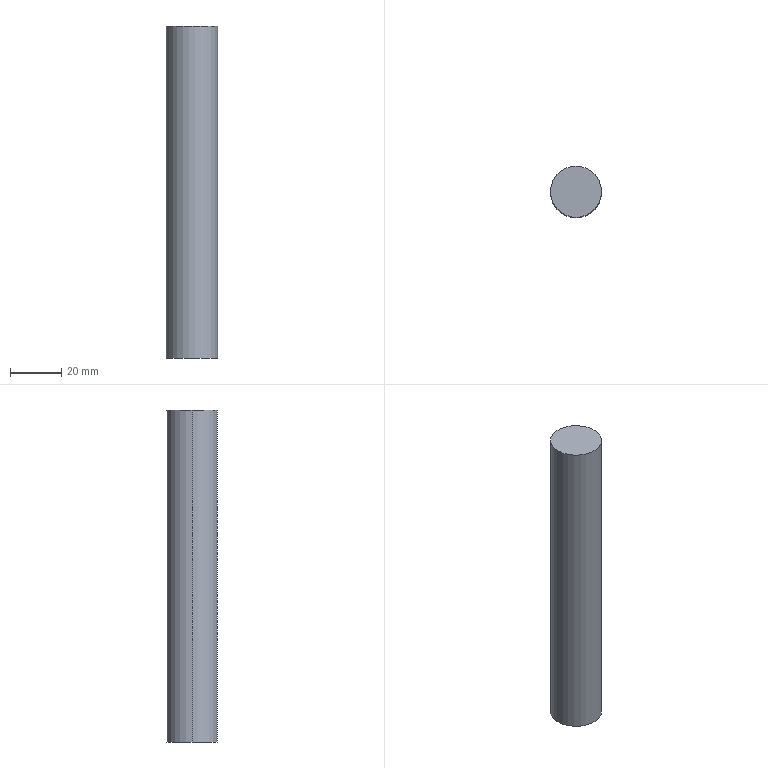Part | SolidWorks | features Extrusion 1 | 1 solid | 4 faces | box 20 x 20 x 130 mm | volume 40841 mm3 | cylinder 2 | plane 2 | commonest cylinder face diameters 20 x2
STEP:
#1=CARTESIAN_POINT('',(10.,0.,130.));
#2=VERTEX_POINT('',#1);
#3=CARTESIAN_POINT('',(-10.,0.,130.));
#4=VERTEX_POINT('',#3);
#5=CARTESIAN_POINT('',(0.,0.,130.));
#6=DIRECTION('',(0.,0.,1.));
#7=DIRECTION('',(1.,0.,0.));
#8=AXIS2_PLACEMENT_3D('',#5,#6,#7);
#9=CIRCLE('',#8,10.);
#10=EDGE_CURVE('',#2,#4,#9,.T.);
#11=ORIENTED_EDGE('',*,*,#10,.F.);
#12=CARTESIAN_POINT('',(10.,0.,0.));
#13=VERTEX_POINT('',#12);
#14=CARTESIAN_POINT('',(10.,0.,130.));
#15=DIRECTION('',(0.,0.,-1.));
#16=VECTOR('',#15,1000.);
#17=LINE('',#14,#16);
#18=EDGE_CURVE('',#2,#13,#17,.T.);
#19=ORIENTED_EDGE('',*,*,#18,.T.);
#20=CARTESIAN_POINT('',(-10.,0.,0.));
#21=VERTEX_POINT('',#20);
#22=CARTESIAN_POINT('',(0.,0.,0.));
#23=DIRECTION('',(0.,0.,1.));
#24=DIRECTION('',(1.,0.,0.));
#25=AXIS2_PLACEMENT_3D('',#22,#23,#24);
#26=CIRCLE('',#25,10.);
#27=EDGE_CURVE('',#13,#21,#26,.T.);
#28=ORIENTED_EDGE('',*,*,#27,.T.);
#29=CARTESIAN_POINT('',(-10.,0.,130.));
#30=DIRECTION('',(0.,0.,-1.));
#31=VECTOR('',#30,1000.);
#32=LINE('',#29,#31);
#33=EDGE_CURVE('',#4,#21,#32,.T.);
#34=ORIENTED_EDGE('',*,*,#33,.F.);
#35=EDGE_LOOP('',(#11,#19,#28,#34));
#36=FACE_OUTER_BOUND('',#35,.T.);
#37=CARTESIAN_POINT('',(0.,0.,130.));
#38=DIRECTION('',(0.,0.,-1.));
#39=DIRECTION('',(-1.,0.,0.));
#40=AXIS2_PLACEMENT_3D('',#37,#38,#39);
#41=CYLINDRICAL_SURFACE('',#40,10.);
#42=ADVANCED_FACE('',(#36),#41,.T.);
#43=ORIENTED_EDGE('',*,*,#18,.F.);
#44=CARTESIAN_POINT('',(0.,0.,130.));
#45=DIRECTION('',(0.,0.,1.));
#46=DIRECTION('',(1.,0.,0.));
#47=AXIS2_PLACEMENT_3D('',#44,#45,#46);
#48=CIRCLE('',#47,10.);
#49=EDGE_CURVE('',#4,#2,#48,.T.);
#50=ORIENTED_EDGE('',*,*,#49,.F.);
#51=ORIENTED_EDGE('',*,*,#33,.T.);
#52=CARTESIAN_POINT('',(0.,0.,0.));
#53=DIRECTION('',(0.,0.,1.));
#54=DIRECTION('',(1.,0.,0.));
#55=AXIS2_PLACEMENT_3D('',#52,#53,#54);
#56=CIRCLE('',#55,10.);
#57=EDGE_CURVE('',#21,#13,#56,.T.);
#58=ORIENTED_EDGE('',*,*,#57,.T.);
#59=EDGE_LOOP('',(#43,#50,#51,#58));
#60=FACE_OUTER_BOUND('',#59,.T.);
#61=CARTESIAN_POINT('',(0.,0.,130.));
#62=DIRECTION('',(0.,0.,-1.));
#63=DIRECTION('',(-1.,0.,0.));
#64=AXIS2_PLACEMENT_3D('',#61,#62,#63);
#65=CYLINDRICAL_SURFACE('',#64,10.);
#66=ADVANCED_FACE('',(#60),#65,.T.);
#67=ORIENTED_EDGE('',*,*,#49,.T.);
#68=ORIENTED_EDGE('',*,*,#10,.T.);
#69=EDGE_LOOP('',(#67,#68));
#70=FACE_OUTER_BOUND('',#69,.T.);
#71=CARTESIAN_POINT('',(0.,0.,130.));
#72=DIRECTION('',(0.,0.,1.));
#73=DIRECTION('',(1.,0.,0.));
#74=AXIS2_PLACEMENT_3D('',#71,#72,#73);
#75=PLANE('',#74);
#76=ADVANCED_FACE('',(#70),#75,.T.);
#77=ORIENTED_EDGE('',*,*,#57,.F.);
#78=ORIENTED_EDGE('',*,*,#27,.F.);
#79=EDGE_LOOP('',(#77,#78));
#80=FACE_OUTER_BOUND('',#79,.T.);
#81=CARTESIAN_POINT('',(0.,0.,0.));
#82=DIRECTION('',(0.,0.,1.));
#83=DIRECTION('',(1.,0.,0.));
#84=AXIS2_PLACEMENT_3D('',#81,#82,#83);
#85=PLANE('',#84);
#86=ADVANCED_FACE('',(#80),#85,.F.);
#87=CLOSED_SHELL('',(#42,#66,#76,#86));
#88=MANIFOLD_SOLID_BREP('',#87);
#89=CARTESIAN_POINT('',(0.,0.,0.));
#90=DIRECTION('',(0.,0.,1.));
#91=DIRECTION('',(1.,0.,0.));
#92=AXIS2_PLACEMENT_3D('',#89,#90,#91);
#93=(LENGTH_UNIT()NAMED_UNIT(*)SI_UNIT(.MILLI.,.METRE.));
#94=UNCERTAINTY_MEASURE_WITH_UNIT(LENGTH_MEASURE(0.00001),#93,'','');
#95=(NAMED_UNIT(*)PLANE_ANGLE_UNIT()SI_UNIT($,.RADIAN.));
#96=(NAMED_UNIT(*)SI_UNIT($,.STERADIAN.)SOLID_ANGLE_UNIT());
#97=(GEOMETRIC_REPRESENTATION_CONTEXT(3)GLOBAL_UNCERTAINTY_ASSIGNED_CONTEXT((#94))GLOBAL_UNIT_ASSIGNED_CONTEXT((#93,#95,#96))REPRESENTATION_CONTEXT('',''));
#98=ADVANCED_BREP_SHAPE_REPRESENTATION('',(#88,#92),#97);